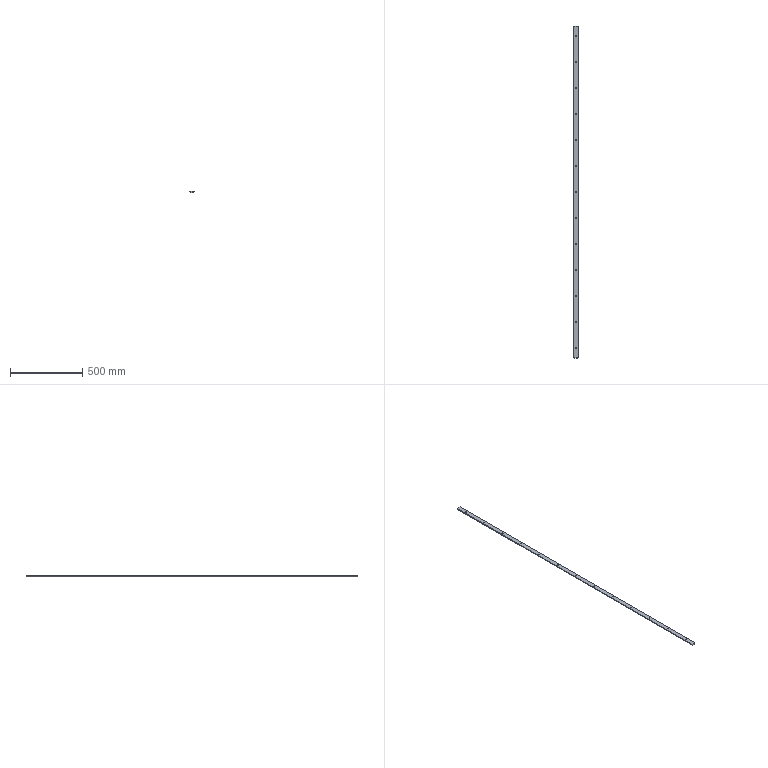Part | NX | features BREP 1 | 1 solid | 73 faces | box 28.8 x 2300 x 11 mm | volume 627359 mm3 | cylinder 52 | plane 21 | commonest cylinder face diameters 5.5 x26 9.5 x26